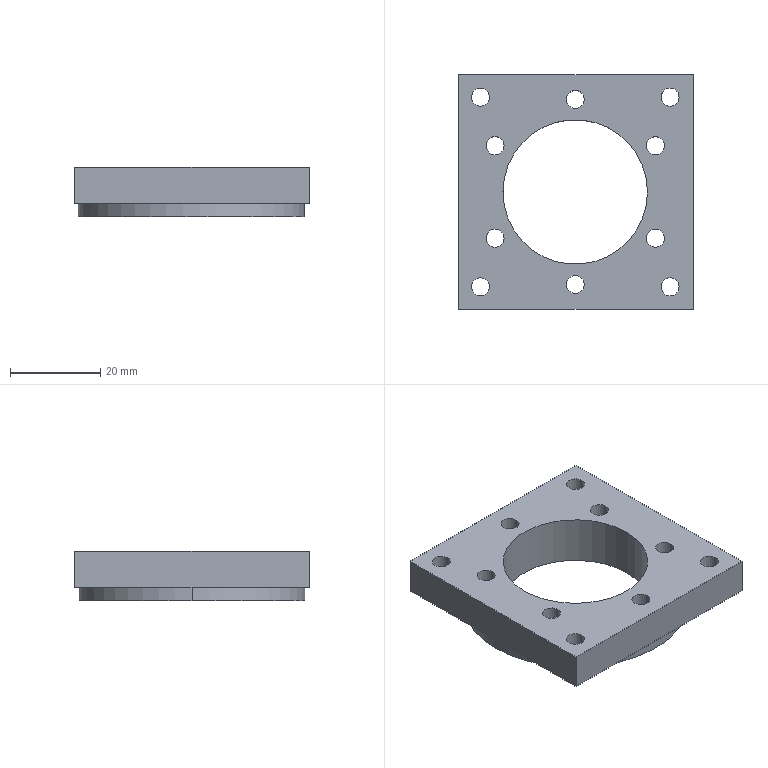Part | SolidWorks | features ICE 4, Extrusion 1 | 1 solid | 49 faces | box 52 x 52 x 11 mm | volume 16978 mm3 | cylinder 36 | plane 13 | commonest cylinder face diameters 4 x20 7 x12 32 x2 50 x2
STEP:
#1=CARTESIAN_POINT('',(-14.254,10.25,3.));
#2=VERTEX_POINT('',#1);
#3=CARTESIAN_POINT('',(-21.254,10.25,3.));
#4=VERTEX_POINT('',#3);
#5=CARTESIAN_POINT('',(-17.754,10.25,3.));
#6=DIRECTION('',(0.,0.,-1.));
#7=DIRECTION('',(-1.,0.,0.));
#8=AXIS2_PLACEMENT_3D('',#5,#6,#7);
#9=CIRCLE('',#8,3.5);
#10=EDGE_CURVE('',#2,#4,#9,.T.);
#11=ORIENTED_EDGE('',*,*,#10,.F.);
#12=CARTESIAN_POINT('',(-14.254,10.25,0.));
#13=VERTEX_POINT('',#12);
#14=CARTESIAN_POINT('',(-14.254,10.25,3.));
#15=DIRECTION('',(0.,0.,-1.));
#16=VECTOR('',#15,1000.);
#17=LINE('',#14,#16);
#18=EDGE_CURVE('',#2,#13,#17,.T.);
#19=ORIENTED_EDGE('',*,*,#18,.T.);
#20=CARTESIAN_POINT('',(-21.254,10.25,0.));
#21=VERTEX_POINT('',#20);
#22=CARTESIAN_POINT('',(-17.754,10.25,0.));
#23=DIRECTION('',(0.,0.,-1.));
#24=DIRECTION('',(-1.,0.,0.));
#25=AXIS2_PLACEMENT_3D('',#22,#23,#24);
#26=CIRCLE('',#25,3.5);
#27=EDGE_CURVE('',#13,#21,#26,.T.);
#28=ORIENTED_EDGE('',*,*,#27,.T.);
#29=CARTESIAN_POINT('',(-21.254,10.25,3.));
#30=DIRECTION('',(0.,0.,-1.));
#31=VECTOR('',#30,1000.);
#32=LINE('',#29,#31);
#33=EDGE_CURVE('',#4,#21,#32,.T.);
#34=ORIENTED_EDGE('',*,*,#33,.F.);
#35=EDGE_LOOP('',(#11,#19,#28,#34));
#36=FACE_OUTER_BOUND('',#35,.T.);
#37=CARTESIAN_POINT('',(-17.754,10.25,3.));
#38=DIRECTION('',(0.,0.,-1.));
#39=DIRECTION('',(-1.,0.,0.));
#40=AXIS2_PLACEMENT_3D('',#37,#38,#39);
#41=CYLINDRICAL_SURFACE('',#40,3.5);
#42=ADVANCED_FACE('',(#36),#41,.F.);
#43=CARTESIAN_POINT('',(-14.254,-10.25,3.));
#44=VERTEX_POINT('',#43);
#45=CARTESIAN_POINT('',(-21.254,-10.25,3.));
#46=VERTEX_POINT('',#45);
#47=CARTESIAN_POINT('',(-17.754,-10.25,3.));
#48=DIRECTION('',(0.,0.,-1.));
#49=DIRECTION('',(-1.,0.,0.));
#50=AXIS2_PLACEMENT_3D('',#47,#48,#49);
#51=CIRCLE('',#50,3.5);
#52=EDGE_CURVE('',#44,#46,#51,.T.);
#53=ORIENTED_EDGE('',*,*,#52,.F.);
#54=CARTESIAN_POINT('',(-14.254,-10.25,0.));
#55=VERTEX_POINT('',#54);
#56=CARTESIAN_POINT('',(-14.254,-10.25,3.));
#57=DIRECTION('',(0.,0.,-1.));
#58=VECTOR('',#57,1000.);
#59=LINE('',#56,#58);
#60=EDGE_CURVE('',#44,#55,#59,.T.);
#61=ORIENTED_EDGE('',*,*,#60,.T.);
#62=CARTESIAN_POINT('',(-21.254,-10.25,0.));
#63=VERTEX_POINT('',#62);
#64=CARTESIAN_POINT('',(-17.754,-10.25,0.));
#65=DIRECTION('',(0.,0.,-1.));
#66=DIRECTION('',(-1.,0.,0.));
#67=AXIS2_PLACEMENT_3D('',#64,#65,#66);
#68=CIRCLE('',#67,3.5);
#69=EDGE_CURVE('',#55,#63,#68,.T.);
#70=ORIENTED_EDGE('',*,*,#69,.T.);
#71=CARTESIAN_POINT('',(-21.254,-10.25,3.));
#72=DIRECTION('',(0.,0.,-1.));
#73=VECTOR('',#72,1000.);
#74=LINE('',#71,#73);
#75=EDGE_CURVE('',#46,#63,#74,.T.);
#76=ORIENTED_EDGE('',*,*,#75,.F.);
#77=EDGE_LOOP('',(#53,#61,#70,#76));
#78=FACE_OUTER_BOUND('',#77,.T.);
#79=CARTESIAN_POINT('',(-17.754,-10.25,3.));
#80=DIRECTION('',(0.,0.,-1.));
#81=DIRECTION('',(-1.,0.,0.));
#82=AXIS2_PLACEMENT_3D('',#79,#80,#81);
#83=CYLINDRICAL_SURFACE('',#82,3.5);
#84=ADVANCED_FACE('',(#78),#83,.F.);
#85=CARTESIAN_POINT('',(3.5,-20.5,3.));
#86=VERTEX_POINT('',#85);
#87=CARTESIAN_POINT('',(-3.5,-20.5,3.));
#88=VERTEX_POINT('',#87);
#89=CARTESIAN_POINT('',(0.,-20.5,3.));
#90=DIRECTION('',(0.,0.,-1.));
#91=DIRECTION('',(-1.,0.,0.));
#92=AXIS2_PLACEMENT_3D('',#89,#90,#91);
#93=CIRCLE('',#92,3.5);
#94=EDGE_CURVE('',#86,#88,#93,.T.);
#95=ORIENTED_EDGE('',*,*,#94,.F.);
#96=CARTESIAN_POINT('',(3.5,-20.5,0.));
#97=VERTEX_POINT('',#96);
#98=CARTESIAN_POINT('',(3.5,-20.5,3.));
#99=DIRECTION('',(0.,0.,-1.));
#100=VECTOR('',#99,1000.);
#101=LINE('',#98,#100);
#102=EDGE_CURVE('',#86,#97,#101,.T.);
#103=ORIENTED_EDGE('',*,*,#102,.T.);
#104=CARTESIAN_POINT('',(-3.5,-20.5,0.));
#105=VERTEX_POINT('',#104);
#106=CARTESIAN_POINT('',(0.,-20.5,0.));
#107=DIRECTION('',(0.,0.,-1.));
#108=DIRECTION('',(-1.,0.,0.));
#109=AXIS2_PLACEMENT_3D('',#106,#107,#108);
#110=CIRCLE('',#109,3.5);
#111=EDGE_CURVE('',#97,#105,#110,.T.);
#112=ORIENTED_EDGE('',*,*,#111,.T.);
#113=CARTESIAN_POINT('',(-3.5,-20.5,3.));
#114=DIRECTION('',(0.,0.,-1.));
#115=VECTOR('',#114,1000.);
#116=LINE('',#113,#115);
#117=EDGE_CURVE('',#88,#105,#116,.T.);
#118=ORIENTED_EDGE('',*,*,#117,.F.);
#119=EDGE_LOOP('',(#95,#103,#112,#118));
#120=FACE_OUTER_BOUND('',#119,.T.);
#121=CARTESIAN_POINT('',(0.,-20.5,3.));
#122=DIRECTION('',(0.,0.,-1.));
#123=DIRECTION('',(-1.,0.,0.));
#124=AXIS2_PLACEMENT_3D('',#121,#122,#123);
#125=CYLINDRICAL_SURFACE('',#124,3.5);
#126=ADVANCED_FACE('',(#120),#125,.F.);
#127=CARTESIAN_POINT('',(21.254,-10.25,3.));
#128=VERTEX_POINT('',#127);
#129=CARTESIAN_POINT('',(14.254,-10.25,3.));
#130=VERTEX_POINT('',#129);
#131=CARTESIAN_POINT('',(17.754,-10.25,3.));
#132=DIRECTION('',(0.,0.,-1.));
#133=DIRECTION('',(-1.,0.,0.));
#134=AXIS2_PLACEMENT_3D('',#131,#132,#133);
#135=CIRCLE('',#134,3.5);
#136=EDGE_CURVE('',#128,#130,#135,.T.);
#137=ORIENTED_EDGE('',*,*,#136,.F.);
#138=CARTESIAN_POINT('',(21.254,-10.25,0.));
#139=VERTEX_POINT('',#138);
#140=CARTESIAN_POINT('',(21.254,-10.25,3.));
#141=DIRECTION('',(0.,0.,-1.));
#142=VECTOR('',#141,1000.);
#143=LINE('',#140,#142);
#144=EDGE_CURVE('',#128,#139,#143,.T.);
#145=ORIENTED_EDGE('',*,*,#144,.T.);
#146=CARTESIAN_POINT('',(14.254,-10.25,0.));
#147=VERTEX_POINT('',#146);
#148=CARTESIAN_POINT('',(17.754,-10.25,0.));
#149=DIRECTION('',(0.,0.,-1.));
#150=DIRECTION('',(-1.,0.,0.));
#151=AXIS2_PLACEMENT_3D('',#148,#149,#150);
#152=CIRCLE('',#151,3.5);
#153=EDGE_CURVE('',#139,#147,#152,.T.);
#154=ORIENTED_EDGE('',*,*,#153,.T.);
#155=CARTESIAN_POINT('',(14.254,-10.25,3.));
#156=DIRECTION('',(0.,0.,-1.));
#157=VECTOR('',#156,1000.);
#158=LINE('',#155,#157);
#159=EDGE_CURVE('',#130,#147,#158,.T.);
#160=ORIENTED_EDGE('',*,*,#159,.F.);
#161=EDGE_LOOP('',(#137,#145,#154,#160));
#162=FACE_OUTER_BOUND('',#161,.T.);
#163=CARTESIAN_POINT('',(17.754,-10.25,3.));
#164=DIRECTION('',(0.,0.,-1.));
#165=DIRECTION('',(-1.,0.,0.));
#166=AXIS2_PLACEMENT_3D('',#163,#164,#165);
#167=CYLINDRICAL_SURFACE('',#166,3.5);
#168=ADVANCED_FACE('',(#162),#167,.F.);
#169=CARTESIAN_POINT('',(21.254,10.25,3.));
#170=VERTEX_POINT('',#169);
#171=CARTESIAN_POINT('',(14.254,10.25,3.));
#172=VERTEX_POINT('',#171);
#173=CARTESIAN_POINT('',(17.754,10.25,3.));
#174=DIRECTION('',(0.,0.,-1.));
#175=DIRECTION('',(-1.,0.,0.));
#176=AXIS2_PLACEMENT_3D('',#173,#174,#175);
#177=CIRCLE('',#176,3.5);
#178=EDGE_CURVE('',#170,#172,#177,.T.);
#179=ORIENTED_EDGE('',*,*,#178,.F.);
#180=CARTESIAN_POINT('',(21.254,10.25,0.));
#181=VERTEX_POINT('',#180);
#182=CARTESIAN_POINT('',(21.254,10.25,3.));
#183=DIRECTION('',(0.,0.,-1.));
#184=VECTOR('',#183,1000.);
#185=LINE('',#182,#184);
#186=EDGE_CURVE('',#170,#181,#185,.T.);
#187=ORIENTED_EDGE('',*,*,#186,.T.);
#188=CARTESIAN_POINT('',(14.254,10.25,0.));
#189=VERTEX_POINT('',#188);
#190=CARTESIAN_POINT('',(17.754,10.25,0.));
#191=DIRECTION('',(0.,0.,-1.));
#192=DIRECTION('',(-1.,0.,0.));
#193=AXIS2_PLACEMENT_3D('',#190,#191,#192);
#194=CIRCLE('',#193,3.5);
#195=EDGE_CURVE('',#181,#189,#194,.T.);
#196=ORIENTED_EDGE('',*,*,#195,.T.);
#197=CARTESIAN_POINT('',(14.254,10.25,3.));
#198=DIRECTION('',(0.,0.,-1.));
#199=VECTOR('',#198,1000.);
#200=LINE('',#197,#199);
#201=EDGE_CURVE('',#172,#189,#200,.T.);
#202=ORIENTED_EDGE('',*,*,#201,.F.);
#203=EDGE_LOOP('',(#179,#187,#196,#202));
#204=FACE_OUTER_BOUND('',#203,.T.);
#205=CARTESIAN_POINT('',(17.754,10.25,3.));
#206=DIRECTION('',(0.,0.,-1.));
#207=DIRECTION('',(-1.,0.,0.));
#208=AXIS2_PLACEMENT_3D('',#205,#206,#207);
#209=CYLINDRICAL_SURFACE('',#208,3.5);
#210=ADVANCED_FACE('',(#204),#209,.F.);
#211=CARTESIAN_POINT('',(3.5,20.5,3.));
#212=VERTEX_POINT('',#211);
#213=CARTESIAN_POINT('',(-3.5,20.5,3.));
#214=VERTEX_POINT('',#213);
#215=CARTESIAN_POINT('',(0.,20.5,3.));
#216=DIRECTION('',(0.,0.,-1.));
#217=DIRECTION('',(-1.,0.,0.));
#218=AXIS2_PLACEMENT_3D('',#215,#216,#217);
#219=CIRCLE('',#218,3.5);
#220=EDGE_CURVE('',#212,#214,#219,.T.);
#221=ORIENTED_EDGE('',*,*,#220,.F.);
#222=CARTESIAN_POINT('',(3.5,20.5,0.));
#223=VERTEX_POINT('',#222);
#224=CARTESIAN_POINT('',(3.5,20.5,3.));
#225=DIRECTION('',(0.,0.,-1.));
#226=VECTOR('',#225,1000.);
#227=LINE('',#224,#226);
#228=EDGE_CURVE('',#212,#223,#227,.T.);
#229=ORIENTED_EDGE('',*,*,#228,.T.);
#230=CARTESIAN_POINT('',(-3.5,20.5,0.));
#231=VERTEX_POINT('',#230);
#232=CARTESIAN_POINT('',(0.,20.5,0.));
#233=DIRECTION('',(0.,0.,-1.));
#234=DIRECTION('',(-1.,0.,0.));
#235=AXIS2_PLACEMENT_3D('',#232,#233,#234);
#236=CIRCLE('',#235,3.5);
#237=EDGE_CURVE('',#223,#231,#236,.T.);
#238=ORIENTED_EDGE('',*,*,#237,.T.);
#239=CARTESIAN_POINT('',(-3.5,20.5,3.));
#240=DIRECTION('',(0.,0.,-1.));
#241=VECTOR('',#240,1000.);
#242=LINE('',#239,#241);
#243=EDGE_CURVE('',#214,#231,#242,.T.);
#244=ORIENTED_EDGE('',*,*,#243,.F.);
#245=EDGE_LOOP('',(#221,#229,#238,#244));
#246=FACE_OUTER_BOUND('',#245,.T.);
#247=CARTESIAN_POINT('',(0.,20.5,3.));
#248=DIRECTION('',(0.,0.,-1.));
#249=DIRECTION('',(-1.,0.,0.));
#250=AXIS2_PLACEMENT_3D('',#247,#248,#249);
#251=CYLINDRICAL_SURFACE('',#250,3.5);
#252=ADVANCED_FACE('',(#246),#251,.F.);
#253=CARTESIAN_POINT('',(23.,-21.,11.));
#254=VERTEX_POINT('',#253);
#255=CARTESIAN_POINT('',(19.,-21.,11.));
#256=VERTEX_POINT('',#255);
#257=CARTESIAN_POINT('',(21.,-21.,11.));
#258=DIRECTION('',(0.,0.,-1.));
#259=DIRECTION('',(1.,0.,0.));
#260=AXIS2_PLACEMENT_3D('',#257,#258,#259);
#261=CIRCLE('',#260,2.);
#262=EDGE_CURVE('',#254,#256,#261,.T.);
#263=ORIENTED_EDGE('',*,*,#262,.F.);
#264=CARTESIAN_POINT('',(23.,-21.,3.));
#265=VERTEX_POINT('',#264);
#266=CARTESIAN_POINT('',(23.,-21.,11.));
#267=DIRECTION('',(0.,0.,-1.));
#268=VECTOR('',#267,1000.);
#269=LINE('',#266,#268);
#270=EDGE_CURVE('',#254,#265,#269,.T.);
#271=ORIENTED_EDGE('',*,*,#270,.T.);
#272=CARTESIAN_POINT('',(19.,-21.,3.));
#273=VERTEX_POINT('',#272);
#274=CARTESIAN_POINT('',(21.,-21.,3.));
#275=DIRECTION('',(0.,0.,-1.));
#276=DIRECTION('',(1.,0.,0.));
#277=AXIS2_PLACEMENT_3D('',#274,#275,#276);
#278=CIRCLE('',#277,2.);
#279=EDGE_CURVE('',#265,#273,#278,.T.);
#280=ORIENTED_EDGE('',*,*,#279,.T.);
#281=CARTESIAN_POINT('',(19.,-21.,11.));
#282=DIRECTION('',(0.,0.,-1.));
#283=VECTOR('',#282,1000.);
#284=LINE('',#281,#283);
#285=EDGE_CURVE('',#256,#273,#284,.T.);
#286=ORIENTED_EDGE('',*,*,#285,.F.);
#287=EDGE_LOOP('',(#263,#271,#280,#286));
#288=FACE_OUTER_BOUND('',#287,.T.);
#289=CARTESIAN_POINT('',(21.,-21.,11.));
#290=DIRECTION('',(0.,0.,-1.));
#291=DIRECTION('',(-1.,0.,0.));
#292=AXIS2_PLACEMENT_3D('',#289,#290,#291);
#293=CYLINDRICAL_SURFACE('',#292,2.);
#294=ADVANCED_FACE('',(#288),#293,.F.);
#295=CARTESIAN_POINT('',(-19.,-21.,11.));
#296=VERTEX_POINT('',#295);
#297=CARTESIAN_POINT('',(-23.,-21.,11.));
#298=VERTEX_POINT('',#297);
#299=CARTESIAN_POINT('',(-21.,-21.,11.));
#300=DIRECTION('',(0.,0.,-1.));
#301=DIRECTION('',(-1.,0.,0.));
#302=AXIS2_PLACEMENT_3D('',#299,#300,#301);
#303=CIRCLE('',#302,2.);
#304=EDGE_CURVE('',#296,#298,#303,.T.);
#305=ORIENTED_EDGE('',*,*,#304,.F.);
#306=CARTESIAN_POINT('',(-19.,-21.,3.));
#307=VERTEX_POINT('',#306);
#308=CARTESIAN_POINT('',(-19.,-21.,11.));
#309=DIRECTION('',(0.,0.,-1.));
#310=VECTOR('',#309,1000.);
#311=LINE('',#308,#310);
#312=EDGE_CURVE('',#296,#307,#311,.T.);
#313=ORIENTED_EDGE('',*,*,#312,.T.);
#314=CARTESIAN_POINT('',(-23.,-21.,3.));
#315=VERTEX_POINT('',#314);
#316=CARTESIAN_POINT('',(-21.,-21.,3.));
#317=DIRECTION('',(0.,0.,-1.));
#318=DIRECTION('',(-1.,0.,0.));
#319=AXIS2_PLACEMENT_3D('',#316,#317,#318);
#320=CIRCLE('',#319,2.);
#321=EDGE_CURVE('',#307,#315,#320,.T.);
#322=ORIENTED_EDGE('',*,*,#321,.T.);
#323=CARTESIAN_POINT('',(-23.,-21.,11.));
#324=DIRECTION('',(0.,0.,-1.));
#325=VECTOR('',#324,1000.);
#326=LINE('',#323,#325);
#327=EDGE_CURVE('',#298,#315,#326,.T.);
#328=ORIENTED_EDGE('',*,*,#327,.F.);
#329=EDGE_LOOP('',(#305,#313,#322,#328));
#330=FACE_OUTER_BOUND('',#329,.T.);
#331=CARTESIAN_POINT('',(-21.,-21.,11.));
#332=DIRECTION('',(0.,0.,-1.));
#333=DIRECTION('',(-1.,0.,0.));
#334=AXIS2_PLACEMENT_3D('',#331,#332,#333);
#335=CYLINDRICAL_SURFACE('',#334,2.);
#336=ADVANCED_FACE('',(#330),#335,.F.);
#337=CARTESIAN_POINT('',(-19.,21.,11.));
#338=VERTEX_POINT('',#337);
#339=CARTESIAN_POINT('',(-23.,21.,11.));
#340=VERTEX_POINT('',#339);
#341=CARTESIAN_POINT('',(-21.,21.,11.));
#342=DIRECTION('',(0.,0.,-1.));
#343=DIRECTION('',(1.,0.,0.));
#344=AXIS2_PLACEMENT_3D('',#341,#342,#343);
#345=CIRCLE('',#344,2.);
#346=EDGE_CURVE('',#338,#340,#345,.T.);
#347=ORIENTED_EDGE('',*,*,#346,.F.);
#348=CARTESIAN_POINT('',(-19.,21.,3.));
#349=VERTEX_POINT('',#348);
#350=CARTESIAN_POINT('',(-19.,21.,11.));
#351=DIRECTION('',(0.,0.,-1.));
#352=VECTOR('',#351,1000.);
#353=LINE('',#350,#352);
#354=EDGE_CURVE('',#338,#349,#353,.T.);
#355=ORIENTED_EDGE('',*,*,#354,.T.);
#356=CARTESIAN_POINT('',(-23.,21.,3.));
#357=VERTEX_POINT('',#356);
#358=CARTESIAN_POINT('',(-21.,21.,3.));
#359=DIRECTION('',(0.,0.,-1.));
#360=DIRECTION('',(1.,0.,0.));
#361=AXIS2_PLACEMENT_3D('',#358,#359,#360);
#362=CIRCLE('',#361,2.);
#363=EDGE_CURVE('',#349,#357,#362,.T.);
#364=ORIENTED_EDGE('',*,*,#363,.T.);
#365=CARTESIAN_POINT('',(-23.,21.,11.));
#366=DIRECTION('',(0.,0.,-1.));
#367=VECTOR('',#366,1000.);
#368=LINE('',#365,#367);
#369=EDGE_CURVE('',#340,#357,#368,.T.);
#370=ORIENTED_EDGE('',*,*,#369,.F.);
#371=EDGE_LOOP('',(#347,#355,#364,#370));
#372=FACE_OUTER_BOUND('',#371,.T.);
#373=CARTESIAN_POINT('',(-21.,21.,11.));
#374=DIRECTION('',(0.,0.,-1.));
#375=DIRECTION('',(-1.,0.,0.));
#376=AXIS2_PLACEMENT_3D('',#373,#374,#375);
#377=CYLINDRICAL_SURFACE('',#376,2.);
#378=ADVANCED_FACE('',(#372),#377,.F.);
#379=CARTESIAN_POINT('',(23.,21.,11.));
#380=VERTEX_POINT('',#379);
#381=CARTESIAN_POINT('',(19.,21.,11.));
#382=VERTEX_POINT('',#381);
#383=CARTESIAN_POINT('',(21.,21.,11.));
#384=DIRECTION('',(0.,0.,-1.));
#385=DIRECTION('',(-1.,0.,0.));
#386=AXIS2_PLACEMENT_3D('',#383,#384,#385);
#387=CIRCLE('',#386,2.);
#388=EDGE_CURVE('',#380,#382,#387,.T.);
#389=ORIENTED_EDGE('',*,*,#388,.F.);
#390=CARTESIAN_POINT('',(23.,21.,3.));
#391=VERTEX_POINT('',#390);
#392=CARTESIAN_POINT('',(23.,21.,11.));
#393=DIRECTION('',(0.,0.,-1.));
#394=VECTOR('',#393,1000.);
#395=LINE('',#392,#394);
#396=EDGE_CURVE('',#380,#391,#395,.T.);
#397=ORIENTED_EDGE('',*,*,#396,.T.);
#398=CARTESIAN_POINT('',(19.,21.,3.));
#399=VERTEX_POINT('',#398);
#400=CARTESIAN_POINT('',(21.,21.,3.));
#401=DIRECTION('',(0.,0.,-1.));
#402=DIRECTION('',(-1.,0.,0.));
#403=AXIS2_PLACEMENT_3D('',#400,#401,#402);
#404=CIRCLE('',#403,2.);
#405=EDGE_CURVE('',#391,#399,#404,.T.);
#406=ORIENTED_EDGE('',*,*,#405,.T.);
#407=CARTESIAN_POINT('',(19.,21.,11.));
#408=DIRECTION('',(0.,0.,-1.));
#409=VECTOR('',#408,1000.);
#410=LINE('',#407,#409);
#411=EDGE_CURVE('',#382,#399,#410,.T.);
#412=ORIENTED_EDGE('',*,*,#411,.F.);
#413=EDGE_LOOP('',(#389,#397,#406,#412));
#414=FACE_OUTER_BOUND('',#413,.T.);
#415=CARTESIAN_POINT('',(21.,21.,11.));
#416=DIRECTION('',(0.,0.,-1.));
#417=DIRECTION('',(-1.,0.,0.));
#418=AXIS2_PLACEMENT_3D('',#415,#416,#417);
#419=CYLINDRICAL_SURFACE('',#418,2.);
#420=ADVANCED_FACE('',(#414),#419,.F.);
#421=CARTESIAN_POINT('',(-16.,0.,11.));
#422=VERTEX_POINT('',#421);
#423=CARTESIAN_POINT('',(16.,0.,11.));
#424=VERTEX_POINT('',#423);
#425=CARTESIAN_POINT('',(0.,0.,11.));
#426=DIRECTION('',(0.,0.,1.));
#427=DIRECTION('',(1.,0.,0.));
#428=AXIS2_PLACEMENT_3D('',#425,#426,#427);
#429=CIRCLE('',#428,16.);
#430=EDGE_CURVE('',#422,#424,#429,.T.);
#431=ORIENTED_EDGE('',*,*,#430,.T.);
#432=CARTESIAN_POINT('',(16.,0.,0.));
#433=VERTEX_POINT('',#432);
#434=CARTESIAN_POINT('',(16.,0.,3.));
#435=DIRECTION('',(0.,0.,-1.));
#436=VECTOR('',#435,1000.);
#437=LINE('',#434,#436);
#438=EDGE_CURVE('',#424,#433,#437,.T.);
#439=ORIENTED_EDGE('',*,*,#438,.T.);
#440=CARTESIAN_POINT('',(-16.,0.,0.));
#441=VERTEX_POINT('',#440);
#442=CARTESIAN_POINT('',(0.,0.,0.));
#443=DIRECTION('',(0.,0.,1.));
#444=DIRECTION('',(1.,0.,0.));
#445=AXIS2_PLACEMENT_3D('',#442,#443,#444);
#446=CIRCLE('',#445,16.);
#447=EDGE_CURVE('',#441,#433,#446,.T.);
#448=ORIENTED_EDGE('',*,*,#447,.F.);
#449=CARTESIAN_POINT('',(-16.,0.,3.));
#450=DIRECTION('',(0.,0.,-1.));
#451=VECTOR('',#450,1000.);
#452=LINE('',#449,#451);
#453=EDGE_CURVE('',#422,#441,#452,.T.);
#454=ORIENTED_EDGE('',*,*,#453,.F.);
#455=EDGE_LOOP('',(#431,#439,#448,#454));
#456=FACE_OUTER_BOUND('',#455,.T.);
#457=CARTESIAN_POINT('',(0.,0.,3.));
#458=DIRECTION('',(0.,0.,-1.));
#459=DIRECTION('',(-1.,0.,0.));
#460=AXIS2_PLACEMENT_3D('',#457,#458,#459);
#461=CYLINDRICAL_SURFACE('',#460,16.);
#462=ADVANCED_FACE('',(#456),#461,.F.);
#463=CARTESIAN_POINT('',(25.,0.,3.));
#464=VERTEX_POINT('',#463);
#465=CARTESIAN_POINT('',(-25.,0.,3.));
#466=VERTEX_POINT('',#465);
#467=CARTESIAN_POINT('',(0.,0.,3.));
#468=DIRECTION('',(0.,0.,1.));
#469=DIRECTION('',(1.,0.,0.));
#470=AXIS2_PLACEMENT_3D('',#467,#468,#469);
#471=CIRCLE('',#470,25.);
#472=EDGE_CURVE('',#464,#466,#471,.T.);
#473=ORIENTED_EDGE('',*,*,#472,.F.);
#474=CARTESIAN_POINT('',(25.,0.,0.));
#475=VERTEX_POINT('',#474);
#476=CARTESIAN_POINT('',(25.,0.,3.));
#477=DIRECTION('',(0.,0.,-1.));
#478=VECTOR('',#477,1000.);
#479=LINE('',#476,#478);
#480=EDGE_CURVE('',#464,#475,#479,.T.);
#481=ORIENTED_EDGE('',*,*,#480,.T.);
#482=CARTESIAN_POINT('',(-25.,0.,0.));
#483=VERTEX_POINT('',#482);
#484=CARTESIAN_POINT('',(0.,0.,0.));
#485=DIRECTION('',(0.,0.,1.));
#486=DIRECTION('',(1.,0.,0.));
#487=AXIS2_PLACEMENT_3D('',#484,#485,#486);
#488=CIRCLE('',#487,25.);
#489=EDGE_CURVE('',#475,#483,#488,.T.);
#490=ORIENTED_EDGE('',*,*,#489,.T.);
#491=CARTESIAN_POINT('',(-25.,0.,3.));
#492=DIRECTION('',(0.,0.,-1.));
#493=VECTOR('',#492,1000.);
#494=LINE('',#491,#493);
#495=EDGE_CURVE('',#466,#483,#494,.T.);
#496=ORIENTED_EDGE('',*,*,#495,.F.);
#497=EDGE_LOOP('',(#473,#481,#490,#496));
#498=FACE_OUTER_BOUND('',#497,.T.);
#499=CARTESIAN_POINT('',(0.,0.,3.));
#500=DIRECTION('',(0.,0.,-1.));
#501=DIRECTION('',(-1.,0.,0.));
#502=AXIS2_PLACEMENT_3D('',#499,#500,#501);
#503=CYLINDRICAL_SURFACE('',#502,25.);
#504=ADVANCED_FACE('',(#498),#503,.T.);
#505=CARTESIAN_POINT('',(2.,20.5,11.));
#506=VERTEX_POINT('',#505);
#507=CARTESIAN_POINT('',(-2.,20.5,11.));
#508=VERTEX_POINT('',#507);
#509=CARTESIAN_POINT('',(0.,20.5,11.));
#510=DIRECTION('',(0.,0.,-1.));
#511=DIRECTION('',(-1.,0.,0.));
#512=AXIS2_PLACEMENT_3D('',#509,#510,#511);
#513=CIRCLE('',#512,2.);
#514=EDGE_CURVE('',#506,#508,#513,.T.);
#515=ORIENTED_EDGE('',*,*,#514,.F.);
#516=CARTESIAN_POINT('',(2.,20.5,3.));
#517=VERTEX_POINT('',#516);
#518=CARTESIAN_POINT('',(2.,20.5,11.));
#519=DIRECTION('',(0.,0.,-1.));
#520=VECTOR('',#519,1000.);
#521=LINE('',#518,#520);
#522=EDGE_CURVE('',#506,#517,#521,.T.);
#523=ORIENTED_EDGE('',*,*,#522,.T.);
#524=CARTESIAN_POINT('',(-2.,20.5,3.));
#525=VERTEX_POINT('',#524);
#526=CARTESIAN_POINT('',(0.,20.5,3.));
#527=DIRECTION('',(0.,0.,1.));
#528=DIRECTION('',(-1.,0.,0.));
#529=AXIS2_PLACEMENT_3D('',#526,#527,#528);
#530=CIRCLE('',#529,2.);
#531=EDGE_CURVE('',#525,#517,#530,.T.);
#532=ORIENTED_EDGE('',*,*,#531,.F.);
#533=CARTESIAN_POINT('',(-2.,20.5,11.));
#534=DIRECTION('',(0.,0.,-1.));
#535=VECTOR('',#534,1000.);
#536=LINE('',#533,#535);
#537=EDGE_CURVE('',#508,#525,#536,.T.);
#538=ORIENTED_EDGE('',*,*,#537,.F.);
#539=EDGE_LOOP('',(#515,#523,#532,#538));
#540=FACE_OUTER_BOUND('',#539,.T.);
#541=CARTESIAN_POINT('',(0.,20.5,11.));
#542=DIRECTION('',(0.,0.,-1.));
#543=DIRECTION('',(-1.,0.,0.));
#544=AXIS2_PLACEMENT_3D('',#541,#542,#543);
#545=CYLINDRICAL_SURFACE('',#544,2.);
#546=ADVANCED_FACE('',(#540),#545,.F.);
#547=CARTESIAN_POINT('',(19.754,10.25,11.));
#548=VERTEX_POINT('',#547);
#549=CARTESIAN_POINT('',(15.754,10.25,11.));
#550=VERTEX_POINT('',#549);
#551=CARTESIAN_POINT('',(17.754,10.25,11.));
#552=DIRECTION('',(0.,0.,-1.));
#553=DIRECTION('',(-1.,0.,0.));
#554=AXIS2_PLACEMENT_3D('',#551,#552,#553);
#555=CIRCLE('',#554,2.);
#556=EDGE_CURVE('',#548,#550,#555,.T.);
#557=ORIENTED_EDGE('',*,*,#556,.F.);
#558=CARTESIAN_POINT('',(19.754,10.25,3.));
#559=VERTEX_POINT('',#558);
#560=CARTESIAN_POINT('',(19.754,10.25,11.));
#561=DIRECTION('',(0.,0.,-1.));
#562=VECTOR('',#561,1000.);
#563=LINE('',#560,#562);
#564=EDGE_CURVE('',#548,#559,#563,.T.);
#565=ORIENTED_EDGE('',*,*,#564,.T.);
#566=CARTESIAN_POINT('',(15.754,10.25,3.));
#567=VERTEX_POINT('',#566);
#568=CARTESIAN_POINT('',(17.754,10.25,3.));
#569=DIRECTION('',(0.,0.,1.));
#570=DIRECTION('',(-1.,0.,0.));
#571=AXIS2_PLACEMENT_3D('',#568,#569,#570);
#572=CIRCLE('',#571,2.);
#573=EDGE_CURVE('',#567,#559,#572,.T.);
#574=ORIENTED_EDGE('',*,*,#573,.F.);
#575=CARTESIAN_POINT('',(15.754,10.25,11.));
#576=DIRECTION('',(0.,0.,-1.));
#577=VECTOR('',#576,1000.);
#578=LINE('',#575,#577);
#579=EDGE_CURVE('',#550,#567,#578,.T.);
#580=ORIENTED_EDGE('',*,*,#579,.F.);
#581=EDGE_LOOP('',(#557,#565,#574,#580));
#582=FACE_OUTER_BOUND('',#581,.T.);
#583=CARTESIAN_POINT('',(17.754,10.25,11.));
#584=DIRECTION('',(0.,0.,-1.));
#585=DIRECTION('',(-1.,0.,0.));
#586=AXIS2_PLACEMENT_3D('',#583,#584,#585);
#587=CYLINDRICAL_SURFACE('',#586,2.);
#588=ADVANCED_FACE('',(#582),#587,.F.);
#589=CARTESIAN_POINT('',(19.754,-10.25,11.));
#590=VERTEX_POINT('',#589);
#591=CARTESIAN_POINT('',(15.754,-10.25,11.));
#592=VERTEX_POINT('',#591);
#593=CARTESIAN_POINT('',(17.754,-10.25,11.));
#594=DIRECTION('',(0.,0.,-1.));
#595=DIRECTION('',(-1.,0.,0.));
#596=AXIS2_PLACEMENT_3D('',#593,#594,#595);
#597=CIRCLE('',#596,2.);
#598=EDGE_CURVE('',#590,#592,#597,.T.);
#599=ORIENTED_EDGE('',*,*,#598,.F.);
#600=CARTESIAN_POINT('',(19.754,-10.25,3.));
#601=VERTEX_POINT('',#600);
#602=CARTESIAN_POINT('',(19.754,-10.25,11.));
#603=DIRECTION('',(0.,0.,-1.));
#604=VECTOR('',#603,1000.);
#605=LINE('',#602,#604);
#606=EDGE_CURVE('',#590,#601,#605,.T.);
#607=ORIENTED_EDGE('',*,*,#606,.T.);
#608=CARTESIAN_POINT('',(15.754,-10.25,3.));
#609=VERTEX_POINT('',#608);
#610=CARTESIAN_POINT('',(17.754,-10.25,3.));
#611=DIRECTION('',(0.,0.,1.));
#612=DIRECTION('',(-1.,0.,0.));
#613=AXIS2_PLACEMENT_3D('',#610,#611,#612);
#614=CIRCLE('',#613,2.);
#615=EDGE_CURVE('',#609,#601,#614,.T.);
#616=ORIENTED_EDGE('',*,*,#615,.F.);
#617=CARTESIAN_POINT('',(15.754,-10.25,11.));
#618=DIRECTION('',(0.,0.,-1.));
#619=VECTOR('',#618,1000.);
#620=LINE('',#617,#619);
#621=EDGE_CURVE('',#592,#609,#620,.T.);
#622=ORIENTED_EDGE('',*,*,#621,.F.);
#623=EDGE_LOOP('',(#599,#607,#616,#622));
#624=FACE_OUTER_BOUND('',#623,.T.);
#625=CARTESIAN_POINT('',(17.754,-10.25,11.));
#626=DIRECTION('',(0.,0.,-1.));
#627=DIRECTION('',(-1.,0.,0.));
#628=AXIS2_PLACEMENT_3D('',#625,#626,#627);
#629=CYLINDRICAL_SURFACE('',#628,2.);
#630=ADVANCED_FACE('',(#624),#629,.F.);
#631=CARTESIAN_POINT('',(2.,-20.5,11.));
#632=VERTEX_POINT('',#631);
#633=CARTESIAN_POINT('',(-2.,-20.5,11.));
#634=VERTEX_POINT('',#633);
#635=CARTESIAN_POINT('',(0.,-20.5,11.));
#636=DIRECTION('',(0.,0.,-1.));
#637=DIRECTION('',(-1.,0.,0.));
#638=AXIS2_PLACEMENT_3D('',#635,#636,#637);
#639=CIRCLE('',#638,2.);
#640=EDGE_CURVE('',#632,#634,#639,.T.);
#641=ORIENTED_EDGE('',*,*,#640,.F.);
#642=CARTESIAN_POINT('',(2.,-20.5,3.));
#643=VERTEX_POINT('',#642);
#644=CARTESIAN_POINT('',(2.,-20.5,11.));
#645=DIRECTION('',(0.,0.,-1.));
#646=VECTOR('',#645,1000.);
#647=LINE('',#644,#646);
#648=EDGE_CURVE('',#632,#643,#647,.T.);
#649=ORIENTED_EDGE('',*,*,#648,.T.);
#650=CARTESIAN_POINT('',(-2.,-20.5,3.));
#651=VERTEX_POINT('',#650);
#652=CARTESIAN_POINT('',(0.,-20.5,3.));
#653=DIRECTION('',(0.,0.,1.));
#654=DIRECTION('',(-1.,0.,0.));
#655=AXIS2_PLACEMENT_3D('',#652,#653,#654);
#656=CIRCLE('',#655,2.);
#657=EDGE_CURVE('',#651,#643,#656,.T.);
#658=ORIENTED_EDGE('',*,*,#657,.F.);
#659=CARTESIAN_POINT('',(-2.,-20.5,11.));
#660=DIRECTION('',(0.,0.,-1.));
#661=VECTOR('',#660,1000.);
#662=LINE('',#659,#661);
#663=EDGE_CURVE('',#634,#651,#662,.T.);
#664=ORIENTED_EDGE('',*,*,#663,.F.);
#665=EDGE_LOOP('',(#641,#649,#658,#664));
#666=FACE_OUTER_BOUND('',#665,.T.);
#667=CARTESIAN_POINT('',(0.,-20.5,11.));
#668=DIRECTION('',(0.,0.,-1.));
#669=DIRECTION('',(-1.,0.,0.));
#670=AXIS2_PLACEMENT_3D('',#667,#668,#669);
#671=CYLINDRICAL_SURFACE('',#670,2.);
#672=ADVANCED_FACE('',(#666),#671,.F.);
#673=CARTESIAN_POINT('',(-15.754,-10.25,11.));
#674=VERTEX_POINT('',#673);
#675=CARTESIAN_POINT('',(-19.754,-10.25,11.));
#676=VERTEX_POINT('',#675);
#677=CARTESIAN_POINT('',(-17.754,-10.25,11.));
#678=DIRECTION('',(0.,0.,-1.));
#679=DIRECTION('',(-1.,0.,0.));
#680=AXIS2_PLACEMENT_3D('',#677,#678,#679);
#681=CIRCLE('',#680,2.);
#682=EDGE_CURVE('',#674,#676,#681,.T.);
#683=ORIENTED_EDGE('',*,*,#682,.F.);
#684=CARTESIAN_POINT('',(-15.754,-10.25,3.));
#685=VERTEX_POINT('',#684);
#686=CARTESIAN_POINT('',(-15.754,-10.25,11.));
#687=DIRECTION('',(0.,0.,-1.));
#688=VECTOR('',#687,1000.);
#689=LINE('',#686,#688);
#690=EDGE_CURVE('',#674,#685,#689,.T.);
#691=ORIENTED_EDGE('',*,*,#690,.T.);
#692=CARTESIAN_POINT('',(-19.754,-10.25,3.));
#693=VERTEX_POINT('',#692);
#694=CARTESIAN_POINT('',(-17.754,-10.25,3.));
#695=DIRECTION('',(0.,0.,1.));
#696=DIRECTION('',(-1.,0.,0.));
#697=AXIS2_PLACEMENT_3D('',#694,#695,#696);
#698=CIRCLE('',#697,2.);
#699=EDGE_CURVE('',#693,#685,#698,.T.);
#700=ORIENTED_EDGE('',*,*,#699,.F.);
#701=CARTESIAN_POINT('',(-19.754,-10.25,11.));
#702=DIRECTION('',(0.,0.,-1.));
#703=VECTOR('',#702,1000.);
#704=LINE('',#701,#703);
#705=EDGE_CURVE('',#676,#693,#704,.T.);
#706=ORIENTED_EDGE('',*,*,#705,.F.);
#707=EDGE_LOOP('',(#683,#691,#700,#706));
#708=FACE_OUTER_BOUND('',#707,.T.);
#709=CARTESIAN_POINT('',(-17.754,-10.25,11.));
#710=DIRECTION('',(0.,0.,-1.));
#711=DIRECTION('',(-1.,0.,0.));
#712=AXIS2_PLACEMENT_3D('',#709,#710,#711);
#713=CYLINDRICAL_SURFACE('',#712,2.);
#714=ADVANCED_FACE('',(#708),#713,.F.);
#715=CARTESIAN_POINT('',(-15.754,10.25,11.));
#716=VERTEX_POINT('',#715);
#717=CARTESIAN_POINT('',(-19.754,10.25,11.));
#718=VERTEX_POINT('',#717);
#719=CARTESIAN_POINT('',(-17.754,10.25,11.));
#720=DIRECTION('',(0.,0.,-1.));
#721=DIRECTION('',(-1.,0.,0.));
#722=AXIS2_PLACEMENT_3D('',#719,#720,#721);
#723=CIRCLE('',#722,2.);
#724=EDGE_CURVE('',#716,#718,#723,.T.);
#725=ORIENTED_EDGE('',*,*,#724,.F.);
#726=CARTESIAN_POINT('',(-15.754,10.25,3.));
#727=VERTEX_POINT('',#726);
#728=CARTESIAN_POINT('',(-15.754,10.25,11.));
#729=DIRECTION('',(0.,0.,-1.));
#730=VECTOR('',#729,1000.);
#731=LINE('',#728,#730);
#732=EDGE_CURVE('',#716,#727,#731,.T.);
#733=ORIENTED_EDGE('',*,*,#732,.T.);
#734=CARTESIAN_POINT('',(-19.754,10.25,3.));
#735=VERTEX_POINT('',#734);
#736=CARTESIAN_POINT('',(-17.754,10.25,3.));
#737=DIRECTION('',(0.,0.,1.));
#738=DIRECTION('',(-1.,0.,0.));
#739=AXIS2_PLACEMENT_3D('',#736,#737,#738);
#740=CIRCLE('',#739,2.);
#741=EDGE_CURVE('',#735,#727,#740,.T.);
#742=ORIENTED_EDGE('',*,*,#741,.F.);
#743=CARTESIAN_POINT('',(-19.754,10.25,11.));
#744=DIRECTION('',(0.,0.,-1.));
#745=VECTOR('',#744,1000.);
#746=LINE('',#743,#745);
#747=EDGE_CURVE('',#718,#735,#746,.T.);
#748=ORIENTED_EDGE('',*,*,#747,.F.);
#749=EDGE_LOOP('',(#725,#733,#742,#748));
#750=FACE_OUTER_BOUND('',#749,.T.);
#751=CARTESIAN_POINT('',(-17.754,10.25,11.));
#752=DIRECTION('',(0.,0.,-1.));
#753=DIRECTION('',(-1.,0.,0.));
#754=AXIS2_PLACEMENT_3D('',#751,#752,#753);
#755=CYLINDRICAL_SURFACE('',#754,2.);
#756=ADVANCED_FACE('',(#750),#755,.F.);
#757=ORIENTED_EDGE('',*,*,#732,.F.);
#758=CARTESIAN_POINT('',(-17.754,10.25,11.));
#759=DIRECTION('',(0.,0.,-1.));
#760=DIRECTION('',(-1.,0.,0.));
#761=AXIS2_PLACEMENT_3D('',#758,#759,#760);
#762=CIRCLE('',#761,2.);
#763=EDGE_CURVE('',#718,#716,#762,.T.);
#764=ORIENTED_EDGE('',*,*,#763,.F.);
#765=ORIENTED_EDGE('',*,*,#747,.T.);
#766=CARTESIAN_POINT('',(-17.754,10.25,3.));
#767=DIRECTION('',(0.,0.,1.));
#768=DIRECTION('',(-1.,0.,0.));
#769=AXIS2_PLACEMENT_3D('',#766,#767,#768);
#770=CIRCLE('',#769,2.);
#771=EDGE_CURVE('',#727,#735,#770,.T.);
#772=ORIENTED_EDGE('',*,*,#771,.F.);
#773=EDGE_LOOP('',(#757,#764,#765,#772));
#774=FACE_OUTER_BOUND('',#773,.T.);
#775=CARTESIAN_POINT('',(-17.754,10.25,11.));
#776=DIRECTION('',(0.,0.,-1.));
#777=DIRECTION('',(-1.,0.,0.));
#778=AXIS2_PLACEMENT_3D('',#775,#776,#777);
#779=CYLINDRICAL_SURFACE('',#778,2.);
#780=ADVANCED_FACE('',(#774),#779,.F.);
#781=ORIENTED_EDGE('',*,*,#690,.F.);
#782=CARTESIAN_POINT('',(-17.754,-10.25,11.));
#783=DIRECTION('',(0.,0.,-1.));
#784=DIRECTION('',(-1.,0.,0.));
#785=AXIS2_PLACEMENT_3D('',#782,#783,#784);
#786=CIRCLE('',#785,2.);
#787=EDGE_CURVE('',#676,#674,#786,.T.);
#788=ORIENTED_EDGE('',*,*,#787,.F.);
#789=ORIENTED_EDGE('',*,*,#705,.T.);
#790=CARTESIAN_POINT('',(-17.754,-10.25,3.));
#791=DIRECTION('',(0.,0.,1.));
#792=DIRECTION('',(-1.,0.,0.));
#793=AXIS2_PLACEMENT_3D('',#790,#791,#792);
#794=CIRCLE('',#793,2.);
#795=EDGE_CURVE('',#685,#693,#794,.T.);
#796=ORIENTED_EDGE('',*,*,#795,.F.);
#797=EDGE_LOOP('',(#781,#788,#789,#796));
#798=FACE_OUTER_BOUND('',#797,.T.);
#799=CARTESIAN_POINT('',(-17.754,-10.25,11.));
#800=DIRECTION('',(0.,0.,-1.));
#801=DIRECTION('',(-1.,0.,0.));
#802=AXIS2_PLACEMENT_3D('',#799,#800,#801);
#803=CYLINDRICAL_SURFACE('',#802,2.);
#804=ADVANCED_FACE('',(#798),#803,.F.);
#805=ORIENTED_EDGE('',*,*,#648,.F.);
#806=CARTESIAN_POINT('',(0.,-20.5,11.));
#807=DIRECTION('',(0.,0.,-1.));
#808=DIRECTION('',(-1.,0.,0.));
#809=AXIS2_PLACEMENT_3D('',#806,#807,#808);
#810=CIRCLE('',#809,2.);
#811=EDGE_CURVE('',#634,#632,#810,.T.);
#812=ORIENTED_EDGE('',*,*,#811,.F.);
#813=ORIENTED_EDGE('',*,*,#663,.T.);
#814=CARTESIAN_POINT('',(0.,-20.5,3.));
#815=DIRECTION('',(0.,0.,1.));
#816=DIRECTION('',(-1.,0.,0.));
#817=AXIS2_PLACEMENT_3D('',#814,#815,#816);
#818=CIRCLE('',#817,2.);
#819=EDGE_CURVE('',#643,#651,#818,.T.);
#820=ORIENTED_EDGE('',*,*,#819,.F.);
#821=EDGE_LOOP('',(#805,#812,#813,#820));
#822=FACE_OUTER_BOUND('',#821,.T.);
#823=CARTESIAN_POINT('',(0.,-20.5,11.));
#824=DIRECTION('',(0.,0.,-1.));
#825=DIRECTION('',(-1.,0.,0.));
#826=AXIS2_PLACEMENT_3D('',#823,#824,#825);
#827=CYLINDRICAL_SURFACE('',#826,2.);
#828=ADVANCED_FACE('',(#822),#827,.F.);
#829=ORIENTED_EDGE('',*,*,#606,.F.);
#830=CARTESIAN_POINT('',(17.754,-10.25,11.));
#831=DIRECTION('',(0.,0.,-1.));
#832=DIRECTION('',(-1.,0.,0.));
#833=AXIS2_PLACEMENT_3D('',#830,#831,#832);
#834=CIRCLE('',#833,2.);
#835=EDGE_CURVE('',#592,#590,#834,.T.);
#836=ORIENTED_EDGE('',*,*,#835,.F.);
#837=ORIENTED_EDGE('',*,*,#621,.T.);
#838=CARTESIAN_POINT('',(17.754,-10.25,3.));
#839=DIRECTION('',(0.,0.,1.));
#840=DIRECTION('',(-1.,0.,0.));
#841=AXIS2_PLACEMENT_3D('',#838,#839,#840);
#842=CIRCLE('',#841,2.);
#843=EDGE_CURVE('',#601,#609,#842,.T.);
#844=ORIENTED_EDGE('',*,*,#843,.F.);
#845=EDGE_LOOP('',(#829,#836,#837,#844));
#846=FACE_OUTER_BOUND('',#845,.T.);
#847=CARTESIAN_POINT('',(17.754,-10.25,11.));
#848=DIRECTION('',(0.,0.,-1.));
#849=DIRECTION('',(-1.,0.,0.));
#850=AXIS2_PLACEMENT_3D('',#847,#848,#849);
#851=CYLINDRICAL_SURFACE('',#850,2.);
#852=ADVANCED_FACE('',(#846),#851,.F.);
#853=ORIENTED_EDGE('',*,*,#564,.F.);
#854=CARTESIAN_POINT('',(17.754,10.25,11.));
#855=DIRECTION('',(0.,0.,-1.));
#856=DIRECTION('',(-1.,0.,0.));
#857=AXIS2_PLACEMENT_3D('',#854,#855,#856);
#858=CIRCLE('',#857,2.);
#859=EDGE_CURVE('',#550,#548,#858,.T.);
#860=ORIENTED_EDGE('',*,*,#859,.F.);
#861=ORIENTED_EDGE('',*,*,#579,.T.);
#862=CARTESIAN_POINT('',(17.754,10.25,3.));
#863=DIRECTION('',(0.,0.,1.));
#864=DIRECTION('',(-1.,0.,0.));
#865=AXIS2_PLACEMENT_3D('',#862,#863,#864);
#866=CIRCLE('',#865,2.);
#867=EDGE_CURVE('',#559,#567,#866,.T.);
#868=ORIENTED_EDGE('',*,*,#867,.F.);
#869=EDGE_LOOP('',(#853,#860,#861,#868));
#870=FACE_OUTER_BOUND('',#869,.T.);
#871=CARTESIAN_POINT('',(17.754,10.25,11.));
#872=DIRECTION('',(0.,0.,-1.));
#873=DIRECTION('',(-1.,0.,0.));
#874=AXIS2_PLACEMENT_3D('',#871,#872,#873);
#875=CYLINDRICAL_SURFACE('',#874,2.);
#876=ADVANCED_FACE('',(#870),#875,.F.);
#877=ORIENTED_EDGE('',*,*,#522,.F.);
#878=CARTESIAN_POINT('',(0.,20.5,11.));
#879=DIRECTION('',(0.,0.,-1.));
#880=DIRECTION('',(-1.,0.,0.));
#881=AXIS2_PLACEMENT_3D('',#878,#879,#880);
#882=CIRCLE('',#881,2.);
#883=EDGE_CURVE('',#508,#506,#882,.T.);
#884=ORIENTED_EDGE('',*,*,#883,.F.);
#885=ORIENTED_EDGE('',*,*,#537,.T.);
#886=CARTESIAN_POINT('',(0.,20.5,3.));
#887=DIRECTION('',(0.,0.,1.));
#888=DIRECTION('',(-1.,0.,0.));
#889=AXIS2_PLACEMENT_3D('',#886,#887,#888);
#890=CIRCLE('',#889,2.);
#891=EDGE_CURVE('',#517,#525,#890,.T.);
#892=ORIENTED_EDGE('',*,*,#891,.F.);
#893=EDGE_LOOP('',(#877,#884,#885,#892));
#894=FACE_OUTER_BOUND('',#893,.T.);
#895=CARTESIAN_POINT('',(0.,20.5,11.));
#896=DIRECTION('',(0.,0.,-1.));
#897=DIRECTION('',(-1.,0.,0.));
#898=AXIS2_PLACEMENT_3D('',#895,#896,#897);
#899=CYLINDRICAL_SURFACE('',#898,2.);
#900=ADVANCED_FACE('',(#894),#899,.F.);
#901=CARTESIAN_POINT('',(0.,20.5,0.));
#902=DIRECTION('',(0.,0.,-1.));
#903=DIRECTION('',(-1.,0.,0.));
#904=AXIS2_PLACEMENT_3D('',#901,#902,#903);
#905=CIRCLE('',#904,3.5);
#906=EDGE_CURVE('',#231,#223,#905,.T.);
#907=ORIENTED_EDGE('',*,*,#906,.F.);
#908=ORIENTED_EDGE('',*,*,#237,.F.);
#909=EDGE_LOOP('',(#907,#908));
#910=FACE_BOUND('',#909,.T.);
#911=CARTESIAN_POINT('',(17.754,10.25,0.));
#912=DIRECTION('',(0.,0.,-1.));
#913=DIRECTION('',(-1.,0.,0.));
#914=AXIS2_PLACEMENT_3D('',#911,#912,#913);
#915=CIRCLE('',#914,3.5);
#916=EDGE_CURVE('',#189,#181,#915,.T.);
#917=ORIENTED_EDGE('',*,*,#916,.F.);
#918=ORIENTED_EDGE('',*,*,#195,.F.);
#919=EDGE_LOOP('',(#917,#918));
#920=FACE_BOUND('',#919,.T.);
#921=CARTESIAN_POINT('',(17.754,-10.25,0.));
#922=DIRECTION('',(0.,0.,-1.));
#923=DIRECTION('',(-1.,0.,0.));
#924=AXIS2_PLACEMENT_3D('',#921,#922,#923);
#925=CIRCLE('',#924,3.5);
#926=EDGE_CURVE('',#147,#139,#925,.T.);
#927=ORIENTED_EDGE('',*,*,#926,.F.);
#928=ORIENTED_EDGE('',*,*,#153,.F.);
#929=EDGE_LOOP('',(#927,#928));
#930=FACE_BOUND('',#929,.T.);
#931=CARTESIAN_POINT('',(0.,-20.5,0.));
#932=DIRECTION('',(0.,0.,-1.));
#933=DIRECTION('',(-1.,0.,0.));
#934=AXIS2_PLACEMENT_3D('',#931,#932,#933);
#935=CIRCLE('',#934,3.5);
#936=EDGE_CURVE('',#105,#97,#935,.T.);
#937=ORIENTED_EDGE('',*,*,#936,.F.);
#938=ORIENTED_EDGE('',*,*,#111,.F.);
#939=EDGE_LOOP('',(#937,#938));
#940=FACE_BOUND('',#939,.T.);
#941=CARTESIAN_POINT('',(-17.754,-10.25,0.));
#942=DIRECTION('',(0.,0.,-1.));
#943=DIRECTION('',(-1.,0.,0.));
#944=AXIS2_PLACEMENT_3D('',#941,#942,#943);
#945=CIRCLE('',#944,3.5);
#946=EDGE_CURVE('',#63,#55,#945,.T.);
#947=ORIENTED_EDGE('',*,*,#946,.F.);
#948=ORIENTED_EDGE('',*,*,#69,.F.);
#949=EDGE_LOOP('',(#947,#948));
#950=FACE_BOUND('',#949,.T.);
#951=CARTESIAN_POINT('',(-17.754,10.25,0.));
#952=DIRECTION('',(0.,0.,-1.));
#953=DIRECTION('',(-1.,0.,0.));
#954=AXIS2_PLACEMENT_3D('',#951,#952,#953);
#955=CIRCLE('',#954,3.5);
#956=EDGE_CURVE('',#21,#13,#955,.T.);
#957=ORIENTED_EDGE('',*,*,#956,.F.);
#958=ORIENTED_EDGE('',*,*,#27,.F.);
#959=EDGE_LOOP('',(#957,#958));
#960=FACE_BOUND('',#959,.T.);
#961=CARTESIAN_POINT('',(0.,0.,0.));
#962=DIRECTION('',(0.,0.,1.));
#963=DIRECTION('',(1.,0.,0.));
#964=AXIS2_PLACEMENT_3D('',#961,#962,#963);
#965=CIRCLE('',#964,25.);
#966=EDGE_CURVE('',#483,#475,#965,.T.);
#967=ORIENTED_EDGE('',*,*,#966,.F.);
#968=ORIENTED_EDGE('',*,*,#489,.F.);
#969=EDGE_LOOP('',(#967,#968));
#970=FACE_OUTER_BOUND('',#969,.T.);
#971=ORIENTED_EDGE('',*,*,#447,.T.);
#972=CARTESIAN_POINT('',(0.,0.,0.));
#973=DIRECTION('',(0.,0.,1.));
#974=DIRECTION('',(1.,0.,0.));
#975=AXIS2_PLACEMENT_3D('',#972,#973,#974);
#976=CIRCLE('',#975,16.);
#977=EDGE_CURVE('',#433,#441,#976,.T.);
#978=ORIENTED_EDGE('',*,*,#977,.T.);
#979=EDGE_LOOP('',(#971,#978));
#980=FACE_BOUND('',#979,.T.);
#981=CARTESIAN_POINT('',(0.,0.,0.));
#982=DIRECTION('',(0.,0.,1.));
#983=DIRECTION('',(1.,0.,0.));
#984=AXIS2_PLACEMENT_3D('',#981,#982,#983);
#985=PLANE('',#984);
#986=ADVANCED_FACE('',(#910,#920,#930,#940,#950,#960,#970,#980),#985,.F.);
#987=ORIENTED_EDGE('',*,*,#480,.F.);
#988=CARTESIAN_POINT('',(0.,0.,3.));
#989=DIRECTION('',(0.,0.,1.));
#990=DIRECTION('',(1.,0.,0.));
#991=AXIS2_PLACEMENT_3D('',#988,#989,#990);
#992=CIRCLE('',#991,25.);
#993=EDGE_CURVE('',#466,#464,#992,.T.);
#994=ORIENTED_EDGE('',*,*,#993,.F.);
#995=ORIENTED_EDGE('',*,*,#495,.T.);
#996=ORIENTED_EDGE('',*,*,#966,.T.);
#997=EDGE_LOOP('',(#987,#994,#995,#996));
#998=FACE_OUTER_BOUND('',#997,.T.);
#999=CARTESIAN_POINT('',(0.,0.,3.));
#1000=DIRECTION('',(0.,0.,-1.));
#1001=DIRECTION('',(-1.,0.,0.));
#1002=AXIS2_PLACEMENT_3D('',#999,#1000,#1001);
#1003=CYLINDRICAL_SURFACE('',#1002,25.);
#1004=ADVANCED_FACE('',(#998),#1003,.T.);
#1005=ORIENTED_EDGE('',*,*,#438,.F.);
#1006=CARTESIAN_POINT('',(0.,0.,11.));
#1007=DIRECTION('',(0.,0.,1.));
#1008=DIRECTION('',(1.,0.,0.));
#1009=AXIS2_PLACEMENT_3D('',#1006,#1007,#1008);
#1010=CIRCLE('',#1009,16.);
#1011=EDGE_CURVE('',#424,#422,#1010,.T.);
#1012=ORIENTED_EDGE('',*,*,#1011,.T.);
#1013=ORIENTED_EDGE('',*,*,#453,.T.);
#1014=ORIENTED_EDGE('',*,*,#977,.F.);
#1015=EDGE_LOOP('',(#1005,#1012,#1013,#1014));
#1016=FACE_OUTER_BOUND('',#1015,.T.);
#1017=CARTESIAN_POINT('',(0.,0.,3.));
#1018=DIRECTION('',(0.,0.,-1.));
#1019=DIRECTION('',(-1.,0.,0.));
#1020=AXIS2_PLACEMENT_3D('',#1017,#1018,#1019);
#1021=CYLINDRICAL_SURFACE('',#1020,16.);
#1022=ADVANCED_FACE('',(#1016),#1021,.F.);
#1023=CARTESIAN_POINT('',(21.,-21.,11.));
#1024=DIRECTION('',(0.,0.,-1.));
#1025=DIRECTION('',(1.,0.,0.));
#1026=AXIS2_PLACEMENT_3D('',#1023,#1024,#1025);
#1027=CIRCLE('',#1026,2.);
#1028=EDGE_CURVE('',#256,#254,#1027,.T.);
#1029=ORIENTED_EDGE('',*,*,#1028,.T.);
#1030=ORIENTED_EDGE('',*,*,#262,.T.);
#1031=EDGE_LOOP('',(#1029,#1030));
#1032=FACE_BOUND('',#1031,.T.);
#1033=CARTESIAN_POINT('',(-21.,-21.,11.));
#1034=DIRECTION('',(0.,0.,-1.));
#1035=DIRECTION('',(-1.,0.,0.));
#1036=AXIS2_PLACEMENT_3D('',#1033,#1034,#1035);
#1037=CIRCLE('',#1036,2.);
#1038=EDGE_CURVE('',#298,#296,#1037,.T.);
#1039=ORIENTED_EDGE('',*,*,#1038,.T.);
#1040=ORIENTED_EDGE('',*,*,#304,.T.);
#1041=EDGE_LOOP('',(#1039,#1040));
#1042=FACE_BOUND('',#1041,.T.);
#1043=CARTESIAN_POINT('',(-21.,21.,11.));
#1044=DIRECTION('',(0.,0.,-1.));
#1045=DIRECTION('',(1.,0.,0.));
#1046=AXIS2_PLACEMENT_3D('',#1043,#1044,#1045);
#1047=CIRCLE('',#1046,2.);
#1048=EDGE_CURVE('',#340,#338,#1047,.T.);
#1049=ORIENTED_EDGE('',*,*,#1048,.T.);
#1050=ORIENTED_EDGE('',*,*,#346,.T.);
#1051=EDGE_LOOP('',(#1049,#1050));
#1052=FACE_BOUND('',#1051,.T.);
#1053=CARTESIAN_POINT('',(21.,21.,11.));
#1054=DIRECTION('',(0.,0.,-1.));
#1055=DIRECTION('',(-1.,0.,0.));
#1056=AXIS2_PLACEMENT_3D('',#1053,#1054,#1055);
#1057=CIRCLE('',#1056,2.);
#1058=EDGE_CURVE('',#382,#380,#1057,.T.);
#1059=ORIENTED_EDGE('',*,*,#1058,.T.);
#1060=ORIENTED_EDGE('',*,*,#388,.T.);
#1061=EDGE_LOOP('',(#1059,#1060));
#1062=FACE_BOUND('',#1061,.T.);
#1063=ORIENTED_EDGE('',*,*,#883,.T.);
#1064=ORIENTED_EDGE('',*,*,#514,.T.);
#1065=EDGE_LOOP('',(#1063,#1064));
#1066=FACE_BOUND('',#1065,.T.);
#1067=ORIENTED_EDGE('',*,*,#859,.T.);
#1068=ORIENTED_EDGE('',*,*,#556,.T.);
#1069=EDGE_LOOP('',(#1067,#1068));
#1070=FACE_BOUND('',#1069,.T.);
#1071=ORIENTED_EDGE('',*,*,#835,.T.);
#1072=ORIENTED_EDGE('',*,*,#598,.T.);
#1073=EDGE_LOOP('',(#1071,#1072));
#1074=FACE_BOUND('',#1073,.T.);
#1075=ORIENTED_EDGE('',*,*,#811,.T.);
#1076=ORIENTED_EDGE('',*,*,#640,.T.);
#1077=EDGE_LOOP('',(#1075,#1076));
#1078=FACE_BOUND('',#1077,.T.);
#1079=ORIENTED_EDGE('',*,*,#787,.T.);
#1080=ORIENTED_EDGE('',*,*,#682,.T.);
#1081=EDGE_LOOP('',(#1079,#1080));
#1082=FACE_BOUND('',#1081,.T.);
#1083=ORIENTED_EDGE('',*,*,#763,.T.);
#1084=ORIENTED_EDGE('',*,*,#724,.T.);
#1085=EDGE_LOOP('',(#1083,#1084));
#1086=FACE_BOUND('',#1085,.T.);
#1087=CARTESIAN_POINT('',(-25.83,26.,11.));
#1088=VERTEX_POINT('',#1087);
#1089=CARTESIAN_POINT('',(-25.83,-26.,11.));
#1090=VERTEX_POINT('',#1089);
#1091=CARTESIAN_POINT('',(-25.83,26.,11.));
#1092=DIRECTION('',(0.,-1.,0.));
#1093=VECTOR('',#1092,1000.);
#1094=LINE('',#1091,#1093);
#1095=EDGE_CURVE('',#1088,#1090,#1094,.T.);
#1096=ORIENTED_EDGE('',*,*,#1095,.T.);
#1097=CARTESIAN_POINT('',(26.17,-26.,11.));
#1098=VERTEX_POINT('',#1097);
#1099=CARTESIAN_POINT('',(-25.83,-26.,11.));
#1100=DIRECTION('',(1.,0.,0.));
#1101=VECTOR('',#1100,1000.);
#1102=LINE('',#1099,#1101);
#1103=EDGE_CURVE('',#1090,#1098,#1102,.T.);
#1104=ORIENTED_EDGE('',*,*,#1103,.T.);
#1105=CARTESIAN_POINT('',(26.17,26.,11.));
#1106=VERTEX_POINT('',#1105);
#1107=CARTESIAN_POINT('',(26.17,26.,11.));
#1108=DIRECTION('',(0.,1.,0.));
#1109=VECTOR('',#1108,1000.);
#1110=LINE('',#1107,#1109);
#1111=EDGE_CURVE('',#1098,#1106,#1110,.T.);
#1112=ORIENTED_EDGE('',*,*,#1111,.T.);
#1113=CARTESIAN_POINT('',(-25.83,26.,11.));
#1114=DIRECTION('',(-1.,0.,0.));
#1115=VECTOR('',#1114,1000.);
#1116=LINE('',#1113,#1115);
#1117=EDGE_CURVE('',#1106,#1088,#1116,.T.);
#1118=ORIENTED_EDGE('',*,*,#1117,.T.);
#1119=EDGE_LOOP('',(#1096,#1104,#1112,#1118));
#1120=FACE_OUTER_BOUND('',#1119,.T.);
#1121=ORIENTED_EDGE('',*,*,#430,.F.);
#1122=ORIENTED_EDGE('',*,*,#1011,.F.);
#1123=EDGE_LOOP('',(#1121,#1122));
#1124=FACE_BOUND('',#1123,.T.);
#1125=CARTESIAN_POINT('',(0.,0.,11.));
#1126=DIRECTION('',(0.,0.,1.));
#1127=DIRECTION('',(1.,0.,0.));
#1128=AXIS2_PLACEMENT_3D('',#1125,#1126,#1127);
#1129=PLANE('',#1128);
#1130=ADVANCED_FACE('',(#1032,#1042,#1052,#1062,#1066,#1070,#1074,#1078,#1082,#1086,#1120,#1124),#1129,.T.);
#1131=CARTESIAN_POINT('',(21.,-21.,3.));
#1132=DIRECTION('',(0.,0.,-1.));
#1133=DIRECTION('',(1.,0.,0.));
#1134=AXIS2_PLACEMENT_3D('',#1131,#1132,#1133);
#1135=CIRCLE('',#1134,2.);
#1136=EDGE_CURVE('',#273,#265,#1135,.T.);
#1137=ORIENTED_EDGE('',*,*,#1136,.F.);
#1138=ORIENTED_EDGE('',*,*,#279,.F.);
#1139=EDGE_LOOP('',(#1137,#1138));
#1140=FACE_BOUND('',#1139,.T.);
#1141=CARTESIAN_POINT('',(-21.,-21.,3.));
#1142=DIRECTION('',(0.,0.,-1.));
#1143=DIRECTION('',(-1.,0.,0.));
#1144=AXIS2_PLACEMENT_3D('',#1141,#1142,#1143);
#1145=CIRCLE('',#1144,2.);
#1146=EDGE_CURVE('',#315,#307,#1145,.T.);
#1147=ORIENTED_EDGE('',*,*,#1146,.F.);
#1148=ORIENTED_EDGE('',*,*,#321,.F.);
#1149=EDGE_LOOP('',(#1147,#1148));
#1150=FACE_BOUND('',#1149,.T.);
#1151=CARTESIAN_POINT('',(-21.,21.,3.));
#1152=DIRECTION('',(0.,0.,-1.));
#1153=DIRECTION('',(1.,0.,0.));
#1154=AXIS2_PLACEMENT_3D('',#1151,#1152,#1153);
#1155=CIRCLE('',#1154,2.);
#1156=EDGE_CURVE('',#357,#349,#1155,.T.);
#1157=ORIENTED_EDGE('',*,*,#1156,.F.);
#1158=ORIENTED_EDGE('',*,*,#363,.F.);
#1159=EDGE_LOOP('',(#1157,#1158));
#1160=FACE_BOUND('',#1159,.T.);
#1161=CARTESIAN_POINT('',(21.,21.,3.));
#1162=DIRECTION('',(0.,0.,-1.));
#1163=DIRECTION('',(-1.,0.,0.));
#1164=AXIS2_PLACEMENT_3D('',#1161,#1162,#1163);
#1165=CIRCLE('',#1164,2.);
#1166=EDGE_CURVE('',#399,#391,#1165,.T.);
#1167=ORIENTED_EDGE('',*,*,#1166,.F.);
#1168=ORIENTED_EDGE('',*,*,#405,.F.);
#1169=EDGE_LOOP('',(#1167,#1168));
#1170=FACE_BOUND('',#1169,.T.);
#1171=ORIENTED_EDGE('',*,*,#993,.T.);
#1172=ORIENTED_EDGE('',*,*,#472,.T.);
#1173=EDGE_LOOP('',(#1171,#1172));
#1174=FACE_BOUND('',#1173,.T.);
#1175=CARTESIAN_POINT('',(-25.83,26.,3.));
#1176=VERTEX_POINT('',#1175);
#1177=CARTESIAN_POINT('',(-25.83,-26.,3.));
#1178=VERTEX_POINT('',#1177);
#1179=CARTESIAN_POINT('',(-25.83,26.,3.));
#1180=DIRECTION('',(0.,-1.,0.));
#1181=VECTOR('',#1180,1000.);
#1182=LINE('',#1179,#1181);
#1183=EDGE_CURVE('',#1176,#1178,#1182,.T.);
#1184=ORIENTED_EDGE('',*,*,#1183,.F.);
#1185=CARTESIAN_POINT('',(26.17,26.,3.));
#1186=VERTEX_POINT('',#1185);
#1187=CARTESIAN_POINT('',(-25.83,26.,3.));
#1188=DIRECTION('',(-1.,0.,0.));
#1189=VECTOR('',#1188,1000.);
#1190=LINE('',#1187,#1189);
#1191=EDGE_CURVE('',#1186,#1176,#1190,.T.);
#1192=ORIENTED_EDGE('',*,*,#1191,.F.);
#1193=CARTESIAN_POINT('',(26.17,-26.,3.));
#1194=VERTEX_POINT('',#1193);
#1195=CARTESIAN_POINT('',(26.17,26.,3.));
#1196=DIRECTION('',(0.,1.,0.));
#1197=VECTOR('',#1196,1000.);
#1198=LINE('',#1195,#1197);
#1199=EDGE_CURVE('',#1194,#1186,#1198,.T.);
#1200=ORIENTED_EDGE('',*,*,#1199,.F.);
#1201=CARTESIAN_POINT('',(-25.83,-26.,3.));
#1202=DIRECTION('',(1.,0.,0.));
#1203=VECTOR('',#1202,1000.);
#1204=LINE('',#1201,#1203);
#1205=EDGE_CURVE('',#1178,#1194,#1204,.T.);
#1206=ORIENTED_EDGE('',*,*,#1205,.F.);
#1207=EDGE_LOOP('',(#1184,#1192,#1200,#1206));
#1208=FACE_OUTER_BOUND('',#1207,.T.);
#1209=CARTESIAN_POINT('',(0.,0.,3.));
#1210=DIRECTION('',(0.,0.,1.));
#1211=DIRECTION('',(1.,0.,0.));
#1212=AXIS2_PLACEMENT_3D('',#1209,#1210,#1211);
#1213=PLANE('',#1212);
#1214=ADVANCED_FACE('',(#1140,#1150,#1160,#1170,#1174,#1208),#1213,.F.);
#1215=ORIENTED_EDGE('',*,*,#1183,.T.);
#1216=CARTESIAN_POINT('',(-25.83,-26.,11.));
#1217=DIRECTION('',(0.,0.,-1.));
#1218=VECTOR('',#1217,1000.);
#1219=LINE('',#1216,#1218);
#1220=EDGE_CURVE('',#1090,#1178,#1219,.T.);
#1221=ORIENTED_EDGE('',*,*,#1220,.F.);
#1222=ORIENTED_EDGE('',*,*,#1095,.F.);
#1223=CARTESIAN_POINT('',(-25.83,26.,11.));
#1224=DIRECTION('',(0.,0.,-1.));
#1225=VECTOR('',#1224,1000.);
#1226=LINE('',#1223,#1225);
#1227=EDGE_CURVE('',#1088,#1176,#1226,.T.);
#1228=ORIENTED_EDGE('',*,*,#1227,.T.);
#1229=EDGE_LOOP('',(#1215,#1221,#1222,#1228));
#1230=FACE_OUTER_BOUND('',#1229,.T.);
#1231=CARTESIAN_POINT('',(-25.83,26.,11.));
#1232=DIRECTION('',(1.,0.,0.));
#1233=DIRECTION('',(0.,0.,-1.));
#1234=AXIS2_PLACEMENT_3D('',#1231,#1232,#1233);
#1235=PLANE('',#1234);
#1236=ADVANCED_FACE('',(#1230),#1235,.F.);
#1237=ORIENTED_EDGE('',*,*,#1205,.T.);
#1238=CARTESIAN_POINT('',(26.17,-26.,11.));
#1239=DIRECTION('',(0.,0.,-1.));
#1240=VECTOR('',#1239,1000.);
#1241=LINE('',#1238,#1240);
#1242=EDGE_CURVE('',#1098,#1194,#1241,.T.);
#1243=ORIENTED_EDGE('',*,*,#1242,.F.);
#1244=ORIENTED_EDGE('',*,*,#1103,.F.);
#1245=ORIENTED_EDGE('',*,*,#1220,.T.);
#1246=EDGE_LOOP('',(#1237,#1243,#1244,#1245));
#1247=FACE_OUTER_BOUND('',#1246,.T.);
#1248=CARTESIAN_POINT('',(-25.83,-26.,11.));
#1249=DIRECTION('',(0.,1.,0.));
#1250=DIRECTION('',(0.,0.,1.));
#1251=AXIS2_PLACEMENT_3D('',#1248,#1249,#1250);
#1252=PLANE('',#1251);
#1253=ADVANCED_FACE('',(#1247),#1252,.F.);
#1254=ORIENTED_EDGE('',*,*,#1199,.T.);
#1255=CARTESIAN_POINT('',(26.17,26.,11.));
#1256=DIRECTION('',(0.,0.,-1.));
#1257=VECTOR('',#1256,1000.);
#1258=LINE('',#1255,#1257);
#1259=EDGE_CURVE('',#1106,#1186,#1258,.T.);
#1260=ORIENTED_EDGE('',*,*,#1259,.F.);
#1261=ORIENTED_EDGE('',*,*,#1111,.F.);
#1262=ORIENTED_EDGE('',*,*,#1242,.T.);
#1263=EDGE_LOOP('',(#1254,#1260,#1261,#1262));
#1264=FACE_OUTER_BOUND('',#1263,.T.);
#1265=CARTESIAN_POINT('',(26.17,26.,11.));
#1266=DIRECTION('',(-1.,0.,0.));
#1267=DIRECTION('',(0.,0.,1.));
#1268=AXIS2_PLACEMENT_3D('',#1265,#1266,#1267);
#1269=PLANE('',#1268);
#1270=ADVANCED_FACE('',(#1264),#1269,.F.);
#1271=ORIENTED_EDGE('',*,*,#1191,.T.);
#1272=ORIENTED_EDGE('',*,*,#1227,.F.);
#1273=ORIENTED_EDGE('',*,*,#1117,.F.);
#1274=ORIENTED_EDGE('',*,*,#1259,.T.);
#1275=EDGE_LOOP('',(#1271,#1272,#1273,#1274));
#1276=FACE_OUTER_BOUND('',#1275,.T.);
#1277=CARTESIAN_POINT('',(-25.83,26.,11.));
#1278=DIRECTION('',(0.,-1.,0.));
#1279=DIRECTION('',(0.,0.,-1.));
#1280=AXIS2_PLACEMENT_3D('',#1277,#1278,#1279);
#1281=PLANE('',#1280);
#1282=ADVANCED_FACE('',(#1276),#1281,.F.);
#1283=ORIENTED_EDGE('',*,*,#396,.F.);
#1284=ORIENTED_EDGE('',*,*,#1058,.F.);
#1285=ORIENTED_EDGE('',*,*,#411,.T.);
#1286=ORIENTED_EDGE('',*,*,#1166,.T.);
#1287=EDGE_LOOP('',(#1283,#1284,#1285,#1286));
#1288=FACE_OUTER_BOUND('',#1287,.T.);
#1289=CARTESIAN_POINT('',(21.,21.,11.));
#1290=DIRECTION('',(0.,0.,-1.));
#1291=DIRECTION('',(-1.,0.,0.));
#1292=AXIS2_PLACEMENT_3D('',#1289,#1290,#1291);
#1293=CYLINDRICAL_SURFACE('',#1292,2.);
#1294=ADVANCED_FACE('',(#1288),#1293,.F.);
#1295=ORIENTED_EDGE('',*,*,#354,.F.);
#1296=ORIENTED_EDGE('',*,*,#1048,.F.);
#1297=ORIENTED_EDGE('',*,*,#369,.T.);
#1298=ORIENTED_EDGE('',*,*,#1156,.T.);
#1299=EDGE_LOOP('',(#1295,#1296,#1297,#1298));
#1300=FACE_OUTER_BOUND('',#1299,.T.);
#1301=CARTESIAN_POINT('',(-21.,21.,11.));
#1302=DIRECTION('',(0.,0.,-1.));
#1303=DIRECTION('',(-1.,0.,0.));
#1304=AXIS2_PLACEMENT_3D('',#1301,#1302,#1303);
#1305=CYLINDRICAL_SURFACE('',#1304,2.);
#1306=ADVANCED_FACE('',(#1300),#1305,.F.);
#1307=ORIENTED_EDGE('',*,*,#312,.F.);
#1308=ORIENTED_EDGE('',*,*,#1038,.F.);
#1309=ORIENTED_EDGE('',*,*,#327,.T.);
#1310=ORIENTED_EDGE('',*,*,#1146,.T.);
#1311=EDGE_LOOP('',(#1307,#1308,#1309,#1310));
#1312=FACE_OUTER_BOUND('',#1311,.T.);
#1313=CARTESIAN_POINT('',(-21.,-21.,11.));
#1314=DIRECTION('',(0.,0.,-1.));
#1315=DIRECTION('',(-1.,0.,0.));
#1316=AXIS2_PLACEMENT_3D('',#1313,#1314,#1315);
#1317=CYLINDRICAL_SURFACE('',#1316,2.);
#1318=ADVANCED_FACE('',(#1312),#1317,.F.);
#1319=ORIENTED_EDGE('',*,*,#270,.F.);
#1320=ORIENTED_EDGE('',*,*,#1028,.F.);
#1321=ORIENTED_EDGE('',*,*,#285,.T.);
#1322=ORIENTED_EDGE('',*,*,#1136,.T.);
#1323=EDGE_LOOP('',(#1319,#1320,#1321,#1322));
#1324=FACE_OUTER_BOUND('',#1323,.T.);
#1325=CARTESIAN_POINT('',(21.,-21.,11.));
#1326=DIRECTION('',(0.,0.,-1.));
#1327=DIRECTION('',(-1.,0.,0.));
#1328=AXIS2_PLACEMENT_3D('',#1325,#1326,#1327);
#1329=CYLINDRICAL_SURFACE('',#1328,2.);
#1330=ADVANCED_FACE('',(#1324),#1329,.F.);
#1331=CARTESIAN_POINT('',(0.,20.5,3.));
#1332=DIRECTION('',(0.,0.,-1.));
#1333=DIRECTION('',(-1.,0.,0.));
#1334=AXIS2_PLACEMENT_3D('',#1331,#1332,#1333);
#1335=CIRCLE('',#1334,3.5);
#1336=EDGE_CURVE('',#214,#212,#1335,.T.);
#1337=ORIENTED_EDGE('',*,*,#1336,.T.);
#1338=ORIENTED_EDGE('',*,*,#220,.T.);
#1339=EDGE_LOOP('',(#1337,#1338));
#1340=FACE_OUTER_BOUND('',#1339,.T.);
#1341=ORIENTED_EDGE('',*,*,#531,.T.);
#1342=ORIENTED_EDGE('',*,*,#891,.T.);
#1343=EDGE_LOOP('',(#1341,#1342));
#1344=FACE_BOUND('',#1343,.T.);
#1345=CARTESIAN_POINT('',(0.,20.5,3.));
#1346=DIRECTION('',(0.,0.,-1.));
#1347=DIRECTION('',(-1.,0.,0.));
#1348=AXIS2_PLACEMENT_3D('',#1345,#1346,#1347);
#1349=PLANE('',#1348);
#1350=ADVANCED_FACE('',(#1340,#1344),#1349,.T.);
#1351=ORIENTED_EDGE('',*,*,#228,.F.);
#1352=ORIENTED_EDGE('',*,*,#1336,.F.);
#1353=ORIENTED_EDGE('',*,*,#243,.T.);
#1354=ORIENTED_EDGE('',*,*,#906,.T.);
#1355=EDGE_LOOP('',(#1351,#1352,#1353,#1354));
#1356=FACE_OUTER_BOUND('',#1355,.T.);
#1357=CARTESIAN_POINT('',(0.,20.5,3.));
#1358=DIRECTION('',(0.,0.,-1.));
#1359=DIRECTION('',(-1.,0.,0.));
#1360=AXIS2_PLACEMENT_3D('',#1357,#1358,#1359);
#1361=CYLINDRICAL_SURFACE('',#1360,3.5);
#1362=ADVANCED_FACE('',(#1356),#1361,.F.);
#1363=CARTESIAN_POINT('',(17.754,10.25,3.));
#1364=DIRECTION('',(0.,0.,-1.));
#1365=DIRECTION('',(-1.,0.,0.));
#1366=AXIS2_PLACEMENT_3D('',#1363,#1364,#1365);
#1367=CIRCLE('',#1366,3.5);
#1368=EDGE_CURVE('',#172,#170,#1367,.T.);
#1369=ORIENTED_EDGE('',*,*,#1368,.T.);
#1370=ORIENTED_EDGE('',*,*,#178,.T.);
#1371=EDGE_LOOP('',(#1369,#1370));
#1372=FACE_OUTER_BOUND('',#1371,.T.);
#1373=ORIENTED_EDGE('',*,*,#573,.T.);
#1374=ORIENTED_EDGE('',*,*,#867,.T.);
#1375=EDGE_LOOP('',(#1373,#1374));
#1376=FACE_BOUND('',#1375,.T.);
#1377=CARTESIAN_POINT('',(17.754,10.25,3.));
#1378=DIRECTION('',(0.,0.,-1.));
#1379=DIRECTION('',(-1.,0.,0.));
#1380=AXIS2_PLACEMENT_3D('',#1377,#1378,#1379);
#1381=PLANE('',#1380);
#1382=ADVANCED_FACE('',(#1372,#1376),#1381,.T.);
#1383=ORIENTED_EDGE('',*,*,#186,.F.);
#1384=ORIENTED_EDGE('',*,*,#1368,.F.);
#1385=ORIENTED_EDGE('',*,*,#201,.T.);
#1386=ORIENTED_EDGE('',*,*,#916,.T.);
#1387=EDGE_LOOP('',(#1383,#1384,#1385,#1386));
#1388=FACE_OUTER_BOUND('',#1387,.T.);
#1389=CARTESIAN_POINT('',(17.754,10.25,3.));
#1390=DIRECTION('',(0.,0.,-1.));
#1391=DIRECTION('',(-1.,0.,0.));
#1392=AXIS2_PLACEMENT_3D('',#1389,#1390,#1391);
#1393=CYLINDRICAL_SURFACE('',#1392,3.5);
#1394=ADVANCED_FACE('',(#1388),#1393,.F.);
#1395=CARTESIAN_POINT('',(17.754,-10.25,3.));
#1396=DIRECTION('',(0.,0.,-1.));
#1397=DIRECTION('',(-1.,0.,0.));
#1398=AXIS2_PLACEMENT_3D('',#1395,#1396,#1397);
#1399=CIRCLE('',#1398,3.5);
#1400=EDGE_CURVE('',#130,#128,#1399,.T.);
#1401=ORIENTED_EDGE('',*,*,#1400,.T.);
#1402=ORIENTED_EDGE('',*,*,#136,.T.);
#1403=EDGE_LOOP('',(#1401,#1402));
#1404=FACE_OUTER_BOUND('',#1403,.T.);
#1405=ORIENTED_EDGE('',*,*,#615,.T.);
#1406=ORIENTED_EDGE('',*,*,#843,.T.);
#1407=EDGE_LOOP('',(#1405,#1406));
#1408=FACE_BOUND('',#1407,.T.);
#1409=CARTESIAN_POINT('',(17.754,-10.25,3.));
#1410=DIRECTION('',(0.,0.,-1.));
#1411=DIRECTION('',(-1.,0.,0.));
#1412=AXIS2_PLACEMENT_3D('',#1409,#1410,#1411);
#1413=PLANE('',#1412);
#1414=ADVANCED_FACE('',(#1404,#1408),#1413,.T.);
#1415=ORIENTED_EDGE('',*,*,#144,.F.);
#1416=ORIENTED_EDGE('',*,*,#1400,.F.);
#1417=ORIENTED_EDGE('',*,*,#159,.T.);
#1418=ORIENTED_EDGE('',*,*,#926,.T.);
#1419=EDGE_LOOP('',(#1415,#1416,#1417,#1418));
#1420=FACE_OUTER_BOUND('',#1419,.T.);
#1421=CARTESIAN_POINT('',(17.754,-10.25,3.));
#1422=DIRECTION('',(0.,0.,-1.));
#1423=DIRECTION('',(-1.,0.,0.));
#1424=AXIS2_PLACEMENT_3D('',#1421,#1422,#1423);
#1425=CYLINDRICAL_SURFACE('',#1424,3.5);
#1426=ADVANCED_FACE('',(#1420),#1425,.F.);
#1427=CARTESIAN_POINT('',(0.,-20.5,3.));
#1428=DIRECTION('',(0.,0.,-1.));
#1429=DIRECTION('',(-1.,0.,0.));
#1430=AXIS2_PLACEMENT_3D('',#1427,#1428,#1429);
#1431=CIRCLE('',#1430,3.5);
#1432=EDGE_CURVE('',#88,#86,#1431,.T.);
#1433=ORIENTED_EDGE('',*,*,#1432,.T.);
#1434=ORIENTED_EDGE('',*,*,#94,.T.);
#1435=EDGE_LOOP('',(#1433,#1434));
#1436=FACE_OUTER_BOUND('',#1435,.T.);
#1437=ORIENTED_EDGE('',*,*,#657,.T.);
#1438=ORIENTED_EDGE('',*,*,#819,.T.);
#1439=EDGE_LOOP('',(#1437,#1438));
#1440=FACE_BOUND('',#1439,.T.);
#1441=CARTESIAN_POINT('',(0.,-20.5,3.));
#1442=DIRECTION('',(0.,0.,-1.));
#1443=DIRECTION('',(-1.,0.,0.));
#1444=AXIS2_PLACEMENT_3D('',#1441,#1442,#1443);
#1445=PLANE('',#1444);
#1446=ADVANCED_FACE('',(#1436,#1440),#1445,.T.);
#1447=ORIENTED_EDGE('',*,*,#102,.F.);
#1448=ORIENTED_EDGE('',*,*,#1432,.F.);
#1449=ORIENTED_EDGE('',*,*,#117,.T.);
#1450=ORIENTED_EDGE('',*,*,#936,.T.);
#1451=EDGE_LOOP('',(#1447,#1448,#1449,#1450));
#1452=FACE_OUTER_BOUND('',#1451,.T.);
#1453=CARTESIAN_POINT('',(0.,-20.5,3.));
#1454=DIRECTION('',(0.,0.,-1.));
#1455=DIRECTION('',(-1.,0.,0.));
#1456=AXIS2_PLACEMENT_3D('',#1453,#1454,#1455);
#1457=CYLINDRICAL_SURFACE('',#1456,3.5);
#1458=ADVANCED_FACE('',(#1452),#1457,.F.);
#1459=CARTESIAN_POINT('',(-17.754,-10.25,3.));
#1460=DIRECTION('',(0.,0.,-1.));
#1461=DIRECTION('',(-1.,0.,0.));
#1462=AXIS2_PLACEMENT_3D('',#1459,#1460,#1461);
#1463=CIRCLE('',#1462,3.5);
#1464=EDGE_CURVE('',#46,#44,#1463,.T.);
#1465=ORIENTED_EDGE('',*,*,#1464,.T.);
#1466=ORIENTED_EDGE('',*,*,#52,.T.);
#1467=EDGE_LOOP('',(#1465,#1466));
#1468=FACE_OUTER_BOUND('',#1467,.T.);
#1469=ORIENTED_EDGE('',*,*,#699,.T.);
#1470=ORIENTED_EDGE('',*,*,#795,.T.);
#1471=EDGE_LOOP('',(#1469,#1470));
#1472=FACE_BOUND('',#1471,.T.);
#1473=CARTESIAN_POINT('',(-17.754,-10.25,3.));
#1474=DIRECTION('',(0.,0.,-1.));
#1475=DIRECTION('',(-1.,0.,0.));
#1476=AXIS2_PLACEMENT_3D('',#1473,#1474,#1475);
#1477=PLANE('',#1476);
#1478=ADVANCED_FACE('',(#1468,#1472),#1477,.T.);
#1479=ORIENTED_EDGE('',*,*,#60,.F.);
#1480=ORIENTED_EDGE('',*,*,#1464,.F.);
#1481=ORIENTED_EDGE('',*,*,#75,.T.);
#1482=ORIENTED_EDGE('',*,*,#946,.T.);
#1483=EDGE_LOOP('',(#1479,#1480,#1481,#1482));
#1484=FACE_OUTER_BOUND('',#1483,.T.);
#1485=CARTESIAN_POINT('',(-17.754,-10.25,3.));
#1486=DIRECTION('',(0.,0.,-1.));
#1487=DIRECTION('',(-1.,0.,0.));
#1488=AXIS2_PLACEMENT_3D('',#1485,#1486,#1487);
#1489=CYLINDRICAL_SURFACE('',#1488,3.5);
#1490=ADVANCED_FACE('',(#1484),#1489,.F.);
#1491=CARTESIAN_POINT('',(-17.754,10.25,3.));
#1492=DIRECTION('',(0.,0.,-1.));
#1493=DIRECTION('',(-1.,0.,0.));
#1494=AXIS2_PLACEMENT_3D('',#1491,#1492,#1493);
#1495=CIRCLE('',#1494,3.5);
#1496=EDGE_CURVE('',#4,#2,#1495,.T.);
#1497=ORIENTED_EDGE('',*,*,#1496,.T.);
#1498=ORIENTED_EDGE('',*,*,#10,.T.);
#1499=EDGE_LOOP('',(#1497,#1498));
#1500=FACE_OUTER_BOUND('',#1499,.T.);
#1501=ORIENTED_EDGE('',*,*,#741,.T.);
#1502=ORIENTED_EDGE('',*,*,#771,.T.);
#1503=EDGE_LOOP('',(#1501,#1502));
#1504=FACE_BOUND('',#1503,.T.);
#1505=CARTESIAN_POINT('',(-17.754,10.25,3.));
#1506=DIRECTION('',(0.,0.,-1.));
#1507=DIRECTION('',(-1.,0.,0.));
#1508=AXIS2_PLACEMENT_3D('',#1505,#1506,#1507);
#1509=PLANE('',#1508);
#1510=ADVANCED_FACE('',(#1500,#1504),#1509,.T.);
#1511=ORIENTED_EDGE('',*,*,#18,.F.);
#1512=ORIENTED_EDGE('',*,*,#1496,.F.);
#1513=ORIENTED_EDGE('',*,*,#33,.T.);
#1514=ORIENTED_EDGE('',*,*,#956,.T.);
#1515=EDGE_LOOP('',(#1511,#1512,#1513,#1514));
#1516=FACE_OUTER_BOUND('',#1515,.T.);
#1517=CARTESIAN_POINT('',(-17.754,10.25,3.));
#1518=DIRECTION('',(0.,0.,-1.));
#1519=DIRECTION('',(-1.,0.,0.));
#1520=AXIS2_PLACEMENT_3D('',#1517,#1518,#1519);
#1521=CYLINDRICAL_SURFACE('',#1520,3.5);
#1522=ADVANCED_FACE('',(#1516),#1521,.F.);
#1523=CLOSED_SHELL('',(#42,#84,#126,#168,#210,#252,#294,#336,#378,#420,#462,#504,#546,#588,#630,#672,#714,#756,#780,#804,#828,#852,#876,#900,#986,#1004,#1022,#1130,#1214,#1236,#1253,#1270,#1282,#1294,#1306,#1318,#1330,#1350,#1362,#1382,#1394,#1414,#1426,#1446,#1458,#1478,#1490,#1510,#1522));
#1524=MANIFOLD_SOLID_BREP('',#1523);
#1525=CARTESIAN_POINT('',(0.,0.,0.));
#1526=DIRECTION('',(0.,0.,1.));
#1527=DIRECTION('',(1.,0.,0.));
#1528=AXIS2_PLACEMENT_3D('',#1525,#1526,#1527);
#1529=(LENGTH_UNIT()NAMED_UNIT(*)SI_UNIT(.MILLI.,.METRE.));
#1530=UNCERTAINTY_MEASURE_WITH_UNIT(LENGTH_MEASURE(0.00001),#1529,'','');
#1531=(NAMED_UNIT(*)PLANE_ANGLE_UNIT()SI_UNIT($,.RADIAN.));
#1532=(NAMED_UNIT(*)SI_UNIT($,.STERADIAN.)SOLID_ANGLE_UNIT());
#1533=(GEOMETRIC_REPRESENTATION_CONTEXT(3)GLOBAL_UNCERTAINTY_ASSIGNED_CONTEXT((#1530))GLOBAL_UNIT_ASSIGNED_CONTEXT((#1529,#1531,#1532))REPRESENTATION_CONTEXT('',''));
#1534=ADVANCED_BREP_SHAPE_REPRESENTATION('',(#1524,#1528),#1533);